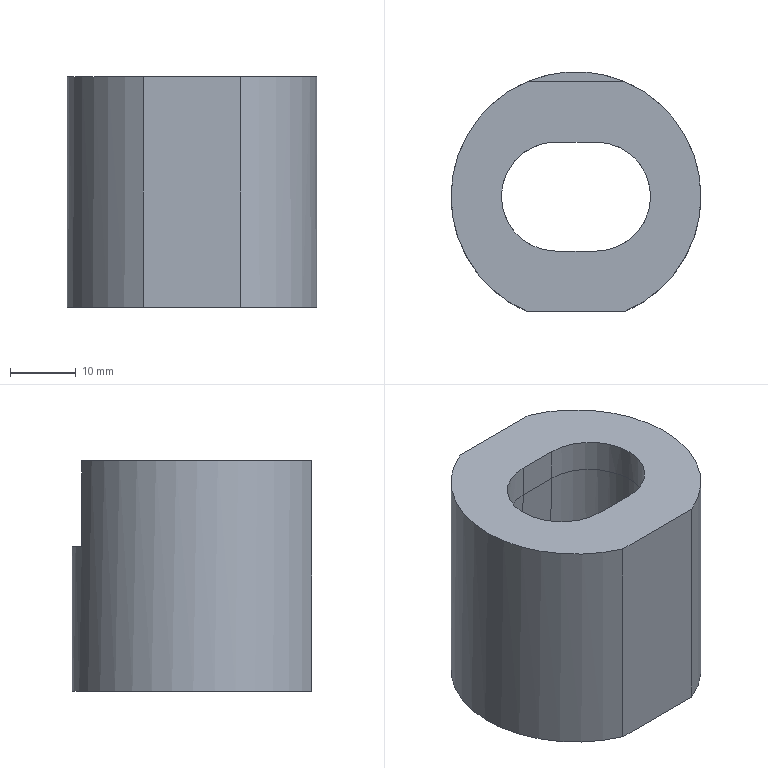Part | STEP file | 1_id4566_x_t | 1 solid | 14 faces | box 38 x 36.5 x 35 mm | volume 27105 mm3 | plane 9 | spline 4 | cylinder 1 | commonest cylinder face diameters 38 x1
STEP:
#1=CARTESIAN_POINT('',(3195.601,138.,-35.));
#2=VERTEX_POINT('',#1);
#3=CARTESIAN_POINT('',(3210.399,138.,-35.));
#4=VERTEX_POINT('',#3);
#5=CARTESIAN_POINT('',(3203.,138.,-35.));
#6=DIRECTION('',(1.,0.,0.));
#7=VECTOR('',#6,1.);
#8=LINE('',#5,#7);
#9=EDGE_CURVE('',#2,#4,#8,.T.);
#10=ORIENTED_EDGE('',*,*,#9,.F.);
#11=CARTESIAN_POINT('',(3203.,155.5,-35.));
#12=DIRECTION('',(0.,0.,1.));
#13=DIRECTION('',(-1.,0.,0.));
#14=AXIS2_PLACEMENT_3D('',#11,#12,#13);
#15=CIRCLE('',#14,19.);
#16=EDGE_CURVE('',#4,#2,#15,.T.);
#17=ORIENTED_EDGE('',*,*,#16,.F.);
#18=EDGE_LOOP('',(#10,#17));
#19=FACE_BOUND('',#18,.T.);
#20=CARTESIAN_POINT('',(3199.935,146.43,-35.));
#21=VERTEX_POINT('',#20);
#22=CARTESIAN_POINT('',(3199.935,164.571,-35.));
#23=VERTEX_POINT('',#22);
#24=CARTESIAN_POINT('',(3199.935,146.43,-35.));
#25=CARTESIAN_POINT('',(3197.549,146.43,-35.));
#26=CARTESIAN_POINT('',(3195.2,147.406,-35.));
#27=CARTESIAN_POINT('',(3191.84,150.768,-35.));
#28=CARTESIAN_POINT('',(3190.867,153.119,-35.));
#29=CARTESIAN_POINT('',(3190.862,157.866,-35.));
#30=CARTESIAN_POINT('',(3191.822,160.211,-35.));
#31=CARTESIAN_POINT('',(3195.207,163.604,-35.));
#32=CARTESIAN_POINT('',(3197.534,164.57,-35.));
#33=CARTESIAN_POINT('',(3199.935,164.571,-35.));
#34=CARTESIAN_POINT('',(3199.935,164.571,-35.));
#35=CARTESIAN_POINT('',(3199.935,164.571,-35.));
#36=B_SPLINE_CURVE_WITH_KNOTS('',3,(#24,#25,#26,#27,#28,#29,#30,#31,#32,#33,#34,#35),.UNSPECIFIED.,.F.,.F.,(4,2,2,2,2,4),(0.,0.25,0.5,0.75,1.,1.),.UNSPECIFIED.);
#37=EDGE_CURVE('',#21,#23,#36,.T.);
#38=ORIENTED_EDGE('',*,*,#37,.F.);
#39=CARTESIAN_POINT('',(3206.065,146.43,-35.));
#40=VERTEX_POINT('',#39);
#41=CARTESIAN_POINT('',(3203.,146.43,-35.));
#42=DIRECTION('',(-1.,0.,0.));
#43=VECTOR('',#42,1.);
#44=LINE('',#41,#43);
#45=EDGE_CURVE('',#40,#21,#44,.T.);
#46=ORIENTED_EDGE('',*,*,#45,.F.);
#47=CARTESIAN_POINT('',(3206.065,164.571,-35.));
#48=VERTEX_POINT('',#47);
#49=CARTESIAN_POINT('',(3206.065,164.571,-35.));
#50=CARTESIAN_POINT('',(3208.452,164.57,-35.));
#51=CARTESIAN_POINT('',(3210.8,163.594,-35.));
#52=CARTESIAN_POINT('',(3214.16,160.233,-35.));
#53=CARTESIAN_POINT('',(3215.134,157.881,-35.));
#54=CARTESIAN_POINT('',(3215.138,153.135,-35.));
#55=CARTESIAN_POINT('',(3214.178,150.789,-35.));
#56=CARTESIAN_POINT('',(3210.793,147.396,-35.));
#57=CARTESIAN_POINT('',(3208.466,146.43,-35.));
#58=CARTESIAN_POINT('',(3206.065,146.43,-35.));
#59=CARTESIAN_POINT('',(3206.065,146.43,-35.));
#60=CARTESIAN_POINT('',(3206.065,146.43,-35.));
#61=B_SPLINE_CURVE_WITH_KNOTS('',3,(#49,#50,#51,#52,#53,#54,#55,#56,#57,#58,#59,#60),.UNSPECIFIED.,.F.,.F.,(4,2,2,2,2,4),(0.,0.25,0.5,0.75,1.,1.),.UNSPECIFIED.);
#62=EDGE_CURVE('',#48,#40,#61,.T.);
#63=ORIENTED_EDGE('',*,*,#62,.F.);
#64=CARTESIAN_POINT('',(3203.,164.571,-35.));
#65=DIRECTION('',(1.,0.,0.));
#66=VECTOR('',#65,1.);
#67=LINE('',#64,#66);
#68=EDGE_CURVE('',#23,#48,#67,.T.);
#69=ORIENTED_EDGE('',*,*,#68,.F.);
#70=EDGE_LOOP('',(#38,#46,#63,#69));
#71=FACE_BOUND('',#70,.T.);
#72=CARTESIAN_POINT('',(3203.,161.75,-35.));
#73=DIRECTION('',(0.,0.,-1.));
#74=DIRECTION('',(0.,1.,0.));
#75=AXIS2_PLACEMENT_3D('',#72,#73,#74);
#76=PLANE('',#75);
#77=ADVANCED_FACE('',(#19,#71),#76,.T.);
#78=CARTESIAN_POINT('',(3195.601,173.,0.00001607));
#79=VERTEX_POINT('',#78);
#80=CARTESIAN_POINT('',(3210.399,173.,0.00001607));
#81=VERTEX_POINT('',#80);
#82=CARTESIAN_POINT('',(3550.42,173.,0.00001607));
#83=DIRECTION('',(1.,0.,0.));
#84=VECTOR('',#83,1.);
#85=LINE('',#82,#84);
#86=EDGE_CURVE('',#79,#81,#85,.T.);
#87=ORIENTED_EDGE('',*,*,#86,.F.);
#88=CARTESIAN_POINT('',(3195.601,138.,0.00001607));
#89=VERTEX_POINT('',#88);
#90=CARTESIAN_POINT('',(3203.,155.5,0.00001607));
#91=DIRECTION('',(0.,0.,1.));
#92=DIRECTION('',(1.,0.,0.));
#93=AXIS2_PLACEMENT_3D('',#90,#91,#92);
#94=CIRCLE('',#93,19.);
#95=EDGE_CURVE('',#79,#89,#94,.T.);
#96=ORIENTED_EDGE('',*,*,#95,.T.);
#97=CARTESIAN_POINT('',(3210.399,138.,0.00001607));
#98=VERTEX_POINT('',#97);
#99=CARTESIAN_POINT('',(3203.,138.,0.00001607));
#100=DIRECTION('',(-1.,0.,0.));
#101=VECTOR('',#100,1.);
#102=LINE('',#99,#101);
#103=EDGE_CURVE('',#98,#89,#102,.T.);
#104=ORIENTED_EDGE('',*,*,#103,.F.);
#105=CARTESIAN_POINT('',(3203.,155.5,0.00001607));
#106=DIRECTION('',(0.,0.,1.));
#107=DIRECTION('',(1.,0.,0.));
#108=AXIS2_PLACEMENT_3D('',#105,#106,#107);
#109=CIRCLE('',#108,19.);
#110=EDGE_CURVE('',#98,#81,#109,.T.);
#111=ORIENTED_EDGE('',*,*,#110,.T.);
#112=EDGE_LOOP('',(#87,#96,#104,#111));
#113=FACE_BOUND('',#112,.T.);
#114=CARTESIAN_POINT('',(3206.065,163.785,0.00001607));
#115=VERTEX_POINT('',#114);
#116=CARTESIAN_POINT('',(3206.065,147.215,0.00001607));
#117=VERTEX_POINT('',#116);
#118=CARTESIAN_POINT('',(3206.065,163.785,0.00001609));
#119=CARTESIAN_POINT('',(3206.589,163.785,0.00001609));
#120=CARTESIAN_POINT('',(3207.146,163.729,0.00001608));
#121=CARTESIAN_POINT('',(3208.207,163.514,0.00001607));
#122=CARTESIAN_POINT('',(3208.728,163.355,0.00001607));
#123=CARTESIAN_POINT('',(3210.231,162.733,0.00001606));
#124=CARTESIAN_POINT('',(3211.155,162.127,0.00001605));
#125=CARTESIAN_POINT('',(3213.46,159.822,0.00001604));
#126=CARTESIAN_POINT('',(3214.35,157.673,0.00001603));
#127=CARTESIAN_POINT('',(3214.35,153.328,0.00001603));
#128=CARTESIAN_POINT('',(3213.46,151.178,0.00001604));
#129=CARTESIAN_POINT('',(3210.387,148.105,0.00001606));
#130=CARTESIAN_POINT('',(3208.228,147.215,0.00001607));
#131=CARTESIAN_POINT('',(3206.065,147.215,0.00001609));
#132=B_SPLINE_CURVE_WITH_KNOTS('',3,(#118,#119,#120,#121,#122,#123,#124,#125,#126,#127,#128,#129,#130,#131),.UNSPECIFIED.,.F.,.F.,(4,2,2,2,2,2,4),(0.,0.0625,0.125,0.25,0.5,0.75,1.),.UNSPECIFIED.);
#133=EDGE_CURVE('',#115,#117,#132,.T.);
#134=ORIENTED_EDGE('',*,*,#133,.T.);
#135=CARTESIAN_POINT('',(3199.935,147.215,0.00001607));
#136=VERTEX_POINT('',#135);
#137=CARTESIAN_POINT('',(3203.,147.215,0.00001607));
#138=DIRECTION('',(-1.,0.,0.));
#139=VECTOR('',#138,1.);
#140=LINE('',#137,#139);
#141=EDGE_CURVE('',#117,#136,#140,.T.);
#142=ORIENTED_EDGE('',*,*,#141,.T.);
#143=CARTESIAN_POINT('',(3199.935,163.785,0.00001607));
#144=VERTEX_POINT('',#143);
#145=CARTESIAN_POINT('',(3199.935,147.215,0.00001607));
#146=CARTESIAN_POINT('',(3197.746,147.215,0.00001607));
#147=CARTESIAN_POINT('',(3195.599,148.119,0.00001607));
#148=CARTESIAN_POINT('',(3192.551,151.168,0.00001607));
#149=CARTESIAN_POINT('',(3191.652,153.333,0.00001607));
#150=CARTESIAN_POINT('',(3191.648,157.654,0.00001607));
#151=CARTESIAN_POINT('',(3192.53,159.809,0.00001607));
#152=CARTESIAN_POINT('',(3195.615,162.9,0.00001607));
#153=CARTESIAN_POINT('',(3197.747,163.785,0.00001607));
#154=CARTESIAN_POINT('',(3199.935,163.785,0.00001607));
#155=B_SPLINE_CURVE_WITH_KNOTS('',3,(#145,#146,#147,#148,#149,#150,#151,#152,#153,#154),.UNSPECIFIED.,.F.,.F.,(4,2,2,2,4),(0.,0.25,0.5,0.75,1.),.UNSPECIFIED.);
#156=EDGE_CURVE('',#136,#144,#155,.T.);
#157=ORIENTED_EDGE('',*,*,#156,.T.);
#158=CARTESIAN_POINT('',(3203.,163.785,0.00001607));
#159=DIRECTION('',(1.,0.,0.));
#160=VECTOR('',#159,1.);
#161=LINE('',#158,#160);
#162=EDGE_CURVE('',#144,#115,#161,.T.);
#163=ORIENTED_EDGE('',*,*,#162,.T.);
#164=EDGE_LOOP('',(#134,#142,#157,#163));
#165=FACE_BOUND('',#164,.T.);
#166=CARTESIAN_POINT('',(3203.,161.75,0.00001607));
#167=DIRECTION('',(0.,0.,1.));
#168=DIRECTION('',(0.,-1.,0.));
#169=AXIS2_PLACEMENT_3D('',#166,#167,#168);
#170=PLANE('',#169);
#171=ADVANCED_FACE('',(#113,#165),#170,.T.);
#172=ORIENTED_EDGE('',*,*,#95,.F.);
#173=CARTESIAN_POINT('',(3195.601,173.,-13.));
#174=VERTEX_POINT('',#173);
#175=CARTESIAN_POINT('',(3195.601,173.,-17.5));
#176=DIRECTION('',(0.,0.,-1.));
#177=VECTOR('',#176,1.);
#178=LINE('',#175,#177);
#179=EDGE_CURVE('',#79,#174,#178,.T.);
#180=ORIENTED_EDGE('',*,*,#179,.T.);
#181=CARTESIAN_POINT('',(3210.399,173.,-13.));
#182=VERTEX_POINT('',#181);
#183=CARTESIAN_POINT('',(3203.,155.5,-13.));
#184=DIRECTION('',(0.,0.,-1.));
#185=DIRECTION('',(1.,0.,0.));
#186=AXIS2_PLACEMENT_3D('',#183,#184,#185);
#187=CIRCLE('',#186,19.);
#188=EDGE_CURVE('',#174,#182,#187,.T.);
#189=ORIENTED_EDGE('',*,*,#188,.T.);
#190=CARTESIAN_POINT('',(3210.399,173.,-17.5));
#191=DIRECTION('',(0.,0.,1.));
#192=VECTOR('',#191,1.);
#193=LINE('',#190,#192);
#194=EDGE_CURVE('',#182,#81,#193,.T.);
#195=ORIENTED_EDGE('',*,*,#194,.T.);
#196=ORIENTED_EDGE('',*,*,#110,.F.);
#197=CARTESIAN_POINT('',(3210.399,138.,-17.5));
#198=DIRECTION('',(0.,0.,1.));
#199=VECTOR('',#198,1.);
#200=LINE('',#197,#199);
#201=EDGE_CURVE('',#4,#98,#200,.T.);
#202=ORIENTED_EDGE('',*,*,#201,.F.);
#203=ORIENTED_EDGE('',*,*,#16,.T.);
#204=CARTESIAN_POINT('',(3195.601,138.,-17.5));
#205=DIRECTION('',(0.,0.,-1.));
#206=VECTOR('',#205,1.);
#207=LINE('',#204,#206);
#208=EDGE_CURVE('',#89,#2,#207,.T.);
#209=ORIENTED_EDGE('',*,*,#208,.F.);
#210=EDGE_LOOP('',(#172,#180,#189,#195,#196,#202,#203,#209));
#211=FACE_OUTER_BOUND('',#210,.T.);
#212=CARTESIAN_POINT('',(3203.,155.5,-17.5));
#213=DIRECTION('',(0.,0.,1.));
#214=DIRECTION('',(0.,-1.,0.));
#215=AXIS2_PLACEMENT_3D('',#212,#213,#214);
#216=CYLINDRICAL_SURFACE('',#215,19.);
#217=ADVANCED_FACE('',(#211),#216,.T.);
#218=CARTESIAN_POINT('',(3199.935,163.785,-5.));
#219=VERTEX_POINT('',#218);
#220=CARTESIAN_POINT('',(3206.065,163.785,-5.));
#221=VERTEX_POINT('',#220);
#222=CARTESIAN_POINT('',(3199.935,163.785,-5.));
#223=DIRECTION('',(1.,0.,0.));
#224=VECTOR('',#223,1.);
#225=LINE('',#222,#224);
#226=EDGE_CURVE('',#219,#221,#225,.T.);
#227=ORIENTED_EDGE('',*,*,#226,.T.);
#228=CARTESIAN_POINT('',(3206.065,163.785,0.00001605));
#229=DIRECTION('',(0.000000008,0.,1.));
#230=VECTOR('',#229,1.);
#231=LINE('',#228,#230);
#232=EDGE_CURVE('',#221,#115,#231,.T.);
#233=ORIENTED_EDGE('',*,*,#232,.T.);
#234=ORIENTED_EDGE('',*,*,#162,.F.);
#235=CARTESIAN_POINT('',(3199.935,163.785,0.0000161));
#236=DIRECTION('',(0.000000008,0.,1.));
#237=VECTOR('',#236,1.);
#238=LINE('',#235,#237);
#239=EDGE_CURVE('',#219,#144,#238,.T.);
#240=ORIENTED_EDGE('',*,*,#239,.F.);
#241=EDGE_LOOP('',(#227,#233,#234,#240));
#242=FACE_OUTER_BOUND('',#241,.T.);
#243=CARTESIAN_POINT('',(3192.,163.785,0.00001616));
#244=DIRECTION('',(0.,-1.,0.));
#245=DIRECTION('',(1.,0.,-0.000000008));
#246=AXIS2_PLACEMENT_3D('',#243,#244,#245);
#247=PLANE('',#246);
#248=ADVANCED_FACE('',(#242),#247,.T.);
#249=CARTESIAN_POINT('',(3199.935,147.215,-5.));
#250=VERTEX_POINT('',#249);
#251=CARTESIAN_POINT('',(3199.926,147.215,-5.));
#252=VERTEX_POINT('',#251);
#253=CARTESIAN_POINT('',(3199.935,147.215,-5.));
#254=CARTESIAN_POINT('',(3199.932,147.215,-5.));
#255=CARTESIAN_POINT('',(3199.929,147.215,-5.));
#256=CARTESIAN_POINT('',(3199.926,147.215,-5.));
#257=B_SPLINE_CURVE_WITH_KNOTS('',3,(#253,#254,#255,#256),.UNSPECIFIED.,.F.,.F.,(4,4),(0.,1.),.UNSPECIFIED.);
#258=EDGE_CURVE('',#250,#252,#257,.T.);
#259=ORIENTED_EDGE('',*,*,#258,.T.);
#260=CARTESIAN_POINT('',(3191.65,155.494,-5.));
#261=VERTEX_POINT('',#260);
#262=CARTESIAN_POINT('',(3199.926,147.215,-5.));
#263=CARTESIAN_POINT('',(3199.334,147.216,-5.));
#264=CARTESIAN_POINT('',(3198.392,147.278,-5.));
#265=CARTESIAN_POINT('',(3196.68,147.868,-5.));
#266=CARTESIAN_POINT('',(3196.057,148.15,-5.));
#267=CARTESIAN_POINT('',(3195.108,148.761,-4.999));
#268=CARTESIAN_POINT('',(3194.76,149.023,-4.999));
#269=CARTESIAN_POINT('',(3194.234,149.478,-5.001));
#270=CARTESIAN_POINT('',(3194.035,149.68,-5.002));
#271=CARTESIAN_POINT('',(3193.741,149.995,-5.007));
#272=CARTESIAN_POINT('',(3193.686,150.057,-5.008));
#273=CARTESIAN_POINT('',(3193.424,150.375,-5.023));
#274=CARTESIAN_POINT('',(3193.266,150.573,-5.034));
#275=CARTESIAN_POINT('',(3192.828,151.234,-5.073));
#276=CARTESIAN_POINT('',(3192.686,151.495,-5.087));
#277=CARTESIAN_POINT('',(3192.505,151.844,-5.101));
#278=CARTESIAN_POINT('',(3192.403,152.055,-5.105));
#279=CARTESIAN_POINT('',(3192.206,152.525,-5.104));
#280=CARTESIAN_POINT('',(3192.111,152.779,-5.099));
#281=CARTESIAN_POINT('',(3191.983,153.192,-5.086));
#282=CARTESIAN_POINT('',(3191.942,153.335,-5.08));
#283=CARTESIAN_POINT('',(3191.867,153.63,-5.067));
#284=CARTESIAN_POINT('',(3191.818,153.85,-5.056));
#285=CARTESIAN_POINT('',(3191.652,154.752,-5.016));
#286=CARTESIAN_POINT('',(3191.65,155.247,-5.));
#287=CARTESIAN_POINT('',(3191.65,155.494,-5.));
#288=B_SPLINE_CURVE_WITH_KNOTS('',3,(#262,#263,#264,#265,#266,#267,#268,#269,#270,#271,#272,#273,#274,#275,#276,#277,#278,#279,#280,#281,#282,#283,#284,#285,#286,#287),.UNSPECIFIED.,.F.,.F.,(4,2,2,2,2,2,2,2,2,2,2,2,4),(0.,0.25,0.375,0.4375,0.5,0.5625,0.625,0.6875,0.75,0.8125,0.8437,0.875,1.),.UNSPECIFIED.);
#289=EDGE_CURVE('',#252,#261,#288,.T.);
#290=ORIENTED_EDGE('',*,*,#289,.T.);
#291=CARTESIAN_POINT('',(3191.991,157.831,-5.));
#292=VERTEX_POINT('',#291);
#293=CARTESIAN_POINT('',(3191.65,155.494,-5.));
#294=CARTESIAN_POINT('',(3191.65,155.496,-5.));
#295=CARTESIAN_POINT('',(3191.65,155.498,-5.));
#296=CARTESIAN_POINT('',(3191.65,156.289,-5.));
#297=CARTESIAN_POINT('',(3191.767,157.076,-5.));
#298=CARTESIAN_POINT('',(3191.991,157.831,-5.));
#299=B_SPLINE_CURVE_WITH_KNOTS('',3,(#293,#294,#295,#296,#297,#298),.UNSPECIFIED.,.F.,.F.,(4,2,4),(0.,0.002603,1.),.UNSPECIFIED.);
#300=EDGE_CURVE('',#261,#292,#299,.T.);
#301=ORIENTED_EDGE('',*,*,#300,.T.);
#302=CARTESIAN_POINT('',(3194.07,161.352,-5.));
#303=VERTEX_POINT('',#302);
#304=CARTESIAN_POINT('',(3191.991,157.831,-5.));
#305=CARTESIAN_POINT('',(3192.381,159.151,-5.));
#306=CARTESIAN_POINT('',(3193.095,160.375,-5.));
#307=CARTESIAN_POINT('',(3194.07,161.352,-5.));
#308=B_SPLINE_CURVE_WITH_KNOTS('',3,(#304,#305,#306,#307),.UNSPECIFIED.,.F.,.F.,(4,4),(0.,1.),.UNSPECIFIED.);
#309=EDGE_CURVE('',#292,#303,#308,.T.);
#310=ORIENTED_EDGE('',*,*,#309,.T.);
#311=CARTESIAN_POINT('',(3199.926,163.785,-5.));
#312=VERTEX_POINT('',#311);
#313=CARTESIAN_POINT('',(3194.07,161.352,-5.));
#314=CARTESIAN_POINT('',(3194.072,161.354,-5.));
#315=CARTESIAN_POINT('',(3194.074,161.356,-5.));
#316=CARTESIAN_POINT('',(3194.845,162.127,-5.));
#317=CARTESIAN_POINT('',(3195.769,162.733,-5.));
#318=CARTESIAN_POINT('',(3197.272,163.355,-5.));
#319=CARTESIAN_POINT('',(3197.793,163.514,-5.));
#320=CARTESIAN_POINT('',(3198.851,163.729,-5.));
#321=CARTESIAN_POINT('',(3199.405,163.784,-5.));
#322=CARTESIAN_POINT('',(3199.926,163.785,-5.));
#323=B_SPLINE_CURVE_WITH_KNOTS('',3,(#313,#314,#315,#316,#317,#318,#319,#320,#321,#322),.UNSPECIFIED.,.F.,.F.,(4,2,2,2,4),(0.,0.001413,0.5014,0.7514,1.),.UNSPECIFIED.);
#324=EDGE_CURVE('',#303,#312,#323,.T.);
#325=ORIENTED_EDGE('',*,*,#324,.T.);
#326=CARTESIAN_POINT('',(3199.926,163.785,-5.));
#327=CARTESIAN_POINT('',(3199.929,163.785,-5.));
#328=CARTESIAN_POINT('',(3199.932,163.785,-5.));
#329=CARTESIAN_POINT('',(3199.935,163.785,-5.));
#330=B_SPLINE_CURVE_WITH_KNOTS('',3,(#326,#327,#328,#329),.UNSPECIFIED.,.F.,.F.,(4,4),(0.,1.),.UNSPECIFIED.);
#331=EDGE_CURVE('',#312,#219,#330,.T.);
#332=ORIENTED_EDGE('',*,*,#331,.T.);
#333=ORIENTED_EDGE('',*,*,#239,.T.);
#334=ORIENTED_EDGE('',*,*,#156,.F.);
#335=CARTESIAN_POINT('',(3199.935,147.215,0.00001609));
#336=DIRECTION('',(0.000000008,0.,1.));
#337=VECTOR('',#336,1.);
#338=LINE('',#335,#337);
#339=EDGE_CURVE('',#250,#136,#338,.T.);
#340=ORIENTED_EDGE('',*,*,#339,.F.);
#341=EDGE_LOOP('',(#259,#290,#301,#310,#325,#332,#333,#334,#340));
#342=FACE_OUTER_BOUND('',#341,.T.);
#343=CARTESIAN_POINT('',(3199.935,147.215,-5.146));
#344=CARTESIAN_POINT('',(3199.935,147.215,0.00001607));
#345=CARTESIAN_POINT('',(3199.411,147.215,-5.146));
#346=CARTESIAN_POINT('',(3199.411,147.215,0.00001608));
#347=CARTESIAN_POINT('',(3198.854,147.271,-5.146));
#348=CARTESIAN_POINT('',(3198.854,147.271,0.00001608));
#349=CARTESIAN_POINT('',(3197.793,147.486,-5.146));
#350=CARTESIAN_POINT('',(3197.793,147.486,0.00001609));
#351=CARTESIAN_POINT('',(3197.272,147.646,-5.146));
#352=CARTESIAN_POINT('',(3197.272,147.646,0.00001609));
#353=CARTESIAN_POINT('',(3195.769,148.267,-5.146));
#354=CARTESIAN_POINT('',(3195.769,148.267,0.0000161));
#355=CARTESIAN_POINT('',(3194.845,148.873,-5.146));
#356=CARTESIAN_POINT('',(3194.845,148.873,0.00001611));
#357=CARTESIAN_POINT('',(3192.54,151.178,-5.146));
#358=CARTESIAN_POINT('',(3192.54,151.178,0.00001613));
#359=CARTESIAN_POINT('',(3191.65,153.327,-5.146));
#360=CARTESIAN_POINT('',(3191.65,153.327,0.00001614));
#361=CARTESIAN_POINT('',(3191.65,157.673,-5.146));
#362=CARTESIAN_POINT('',(3191.65,157.673,0.00001614));
#363=CARTESIAN_POINT('',(3192.54,159.822,-5.146));
#364=CARTESIAN_POINT('',(3192.54,159.822,0.00001613));
#365=CARTESIAN_POINT('',(3194.845,162.127,-5.146));
#366=CARTESIAN_POINT('',(3194.845,162.127,0.00001611));
#367=CARTESIAN_POINT('',(3195.769,162.733,-5.146));
#368=CARTESIAN_POINT('',(3195.769,162.733,0.0000161));
#369=CARTESIAN_POINT('',(3197.272,163.355,-5.146));
#370=CARTESIAN_POINT('',(3197.272,163.355,0.00001609));
#371=CARTESIAN_POINT('',(3197.793,163.514,-5.146));
#372=CARTESIAN_POINT('',(3197.793,163.514,0.00001609));
#373=CARTESIAN_POINT('',(3198.854,163.729,-5.146));
#374=CARTESIAN_POINT('',(3198.854,163.729,0.00001608));
#375=CARTESIAN_POINT('',(3199.411,163.785,-5.146));
#376=CARTESIAN_POINT('',(3199.411,163.785,0.00001608));
#377=CARTESIAN_POINT('',(3199.935,163.785,-5.146));
#378=CARTESIAN_POINT('',(3199.935,163.785,0.00001607));
#379=B_SPLINE_SURFACE_WITH_KNOTS('',3,1,((#343,#344),(#345,#346),(#347,#348),(#349,#350),(#351,#352),(#353,#354),(#355,#356),(#357,#358),(#359,#360),(#361,#362),(#363,#364),(#365,#366),(#367,#368),(#369,#370),(#371,#372),(#373,#374),(#375,#376),(#377,#378)),.UNSPECIFIED.,.F.,.F.,.F.,(4,2,2,2,2,2,2,2,4),(2,2),(0.,0.0625,0.125,0.25,0.5,0.75,0.875,0.9375,1.),(0.,1.),.UNSPECIFIED.);
#380=ADVANCED_FACE('',(#342),#379,.T.);
#381=CARTESIAN_POINT('',(3206.075,163.785,-5.));
#382=VERTEX_POINT('',#381);
#383=CARTESIAN_POINT('',(3206.07,163.785,-5.));
#384=DIRECTION('',(1.,-0.0001546,0.));
#385=VECTOR('',#384,1.);
#386=LINE('',#383,#385);
#387=EDGE_CURVE('',#221,#382,#386,.T.);
#388=ORIENTED_EDGE('',*,*,#387,.T.);
#389=CARTESIAN_POINT('',(3214.35,155.507,-5.));
#390=VERTEX_POINT('',#389);
#391=CARTESIAN_POINT('',(3206.075,163.785,-5.));
#392=CARTESIAN_POINT('',(3208.263,163.782,-5.));
#393=CARTESIAN_POINT('',(3210.406,162.88,-4.999));
#394=CARTESIAN_POINT('',(3212.692,160.588,-5.001));
#395=CARTESIAN_POINT('',(3213.3,159.663,-5.107));
#396=CARTESIAN_POINT('',(3214.125,157.671,-5.107));
#397=CARTESIAN_POINT('',(3214.349,156.587,-5.));
#398=CARTESIAN_POINT('',(3214.35,155.507,-5.));
#399=B_SPLINE_CURVE_WITH_KNOTS('',3,(#391,#392,#393,#394,#395,#396,#397,#398),.UNSPECIFIED.,.F.,.F.,(4,2,2,4),(0.,0.5,0.75,1.),.UNSPECIFIED.);
#400=EDGE_CURVE('',#382,#390,#399,.T.);
#401=ORIENTED_EDGE('',*,*,#400,.T.);
#402=CARTESIAN_POINT('',(3214.35,155.506,-5.));
#403=VERTEX_POINT('',#402);
#404=CARTESIAN_POINT('',(3214.35,155.507,-5.));
#405=CARTESIAN_POINT('',(3214.35,155.507,-5.));
#406=CARTESIAN_POINT('',(3214.35,155.507,-5.));
#407=CARTESIAN_POINT('',(3214.35,155.506,-5.));
#408=B_SPLINE_CURVE_WITH_KNOTS('',3,(#404,#405,#406,#407),.UNSPECIFIED.,.F.,.F.,(4,4),(0.,1.),.UNSPECIFIED.);
#409=EDGE_CURVE('',#390,#403,#408,.T.);
#410=ORIENTED_EDGE('',*,*,#409,.T.);
#411=CARTESIAN_POINT('',(3214.009,153.171,-5.));
#412=VERTEX_POINT('',#411);
#413=CARTESIAN_POINT('',(3214.35,155.506,-5.));
#414=CARTESIAN_POINT('',(3214.351,154.715,-5.));
#415=CARTESIAN_POINT('',(3214.233,153.926,-5.002));
#416=CARTESIAN_POINT('',(3214.01,153.17,-5.));
#417=B_SPLINE_CURVE_WITH_KNOTS('',3,(#413,#414,#415,#416),.UNSPECIFIED.,.F.,.F.,(4,4),(0.,1.),.UNSPECIFIED.);
#418=EDGE_CURVE('',#403,#412,#417,.T.);
#419=ORIENTED_EDGE('',*,*,#418,.T.);
#420=CARTESIAN_POINT('',(3211.93,149.648,-5.));
#421=VERTEX_POINT('',#420);
#422=CARTESIAN_POINT('',(3214.01,153.17,-5.));
#423=CARTESIAN_POINT('',(3213.619,151.85,-5.));
#424=CARTESIAN_POINT('',(3212.905,150.626,-5.));
#425=CARTESIAN_POINT('',(3211.93,149.648,-5.));
#426=B_SPLINE_CURVE_WITH_KNOTS('',3,(#422,#423,#424,#425),.UNSPECIFIED.,.F.,.F.,(4,4),(0.,1.),.UNSPECIFIED.);
#427=EDGE_CURVE('',#412,#421,#426,.T.);
#428=ORIENTED_EDGE('',*,*,#427,.T.);
#429=CARTESIAN_POINT('',(3206.074,147.215,-5.));
#430=VERTEX_POINT('',#429);
#431=CARTESIAN_POINT('',(3211.93,149.648,-5.));
#432=CARTESIAN_POINT('',(3211.928,149.646,-5.));
#433=CARTESIAN_POINT('',(3211.926,149.644,-5.));
#434=CARTESIAN_POINT('',(3210.389,148.108,-5.));
#435=CARTESIAN_POINT('',(3208.234,147.218,-5.));
#436=CARTESIAN_POINT('',(3206.074,147.215,-5.));
#437=B_SPLINE_CURVE_WITH_KNOTS('',3,(#431,#432,#433,#434,#435,#436),.UNSPECIFIED.,.F.,.F.,(4,2,4),(0.,0.00141,1.),.UNSPECIFIED.);
#438=EDGE_CURVE('',#421,#430,#437,.T.);
#439=ORIENTED_EDGE('',*,*,#438,.T.);
#440=CARTESIAN_POINT('',(3206.065,147.215,-5.));
#441=VERTEX_POINT('',#440);
#442=CARTESIAN_POINT('',(3206.074,147.215,-5.));
#443=CARTESIAN_POINT('',(3206.071,147.215,-5.));
#444=CARTESIAN_POINT('',(3206.068,147.215,-5.));
#445=CARTESIAN_POINT('',(3206.065,147.215,-5.));
#446=B_SPLINE_CURVE_WITH_KNOTS('',3,(#442,#443,#444,#445),.UNSPECIFIED.,.F.,.F.,(4,4),(0.,1.),.UNSPECIFIED.);
#447=EDGE_CURVE('',#430,#441,#446,.T.);
#448=ORIENTED_EDGE('',*,*,#447,.T.);
#449=CARTESIAN_POINT('',(3206.065,147.215,0.00001605));
#450=DIRECTION('',(0.000000008,0.,1.));
#451=VECTOR('',#450,1.);
#452=LINE('',#449,#451);
#453=EDGE_CURVE('',#441,#117,#452,.T.);
#454=ORIENTED_EDGE('',*,*,#453,.T.);
#455=ORIENTED_EDGE('',*,*,#133,.F.);
#456=ORIENTED_EDGE('',*,*,#232,.F.);
#457=EDGE_LOOP('',(#388,#401,#410,#419,#428,#439,#448,#454,#455,#456));
#458=FACE_OUTER_BOUND('',#457,.T.);
#459=CARTESIAN_POINT('',(3206.065,163.785,-5.146));
#460=CARTESIAN_POINT('',(3206.065,163.785,0.0000161));
#461=CARTESIAN_POINT('',(3206.589,163.785,-5.146));
#462=CARTESIAN_POINT('',(3206.589,163.785,0.0000161));
#463=CARTESIAN_POINT('',(3207.146,163.729,-5.146));
#464=CARTESIAN_POINT('',(3207.146,163.729,0.0000161));
#465=CARTESIAN_POINT('',(3208.207,163.514,-5.146));
#466=CARTESIAN_POINT('',(3208.207,163.514,0.00001609));
#467=CARTESIAN_POINT('',(3208.728,163.355,-5.146));
#468=CARTESIAN_POINT('',(3208.728,163.355,0.00001608));
#469=CARTESIAN_POINT('',(3210.231,162.733,-5.146));
#470=CARTESIAN_POINT('',(3210.231,162.733,0.00001607));
#471=CARTESIAN_POINT('',(3211.155,162.127,-5.146));
#472=CARTESIAN_POINT('',(3211.155,162.127,0.00001607));
#473=CARTESIAN_POINT('',(3213.46,159.822,-5.146));
#474=CARTESIAN_POINT('',(3213.46,159.822,0.00001605));
#475=CARTESIAN_POINT('',(3214.35,157.673,-5.146));
#476=CARTESIAN_POINT('',(3214.35,157.673,0.00001604));
#477=CARTESIAN_POINT('',(3214.35,153.328,-5.146));
#478=CARTESIAN_POINT('',(3214.35,153.328,0.00001604));
#479=CARTESIAN_POINT('',(3213.46,151.178,-5.146));
#480=CARTESIAN_POINT('',(3213.46,151.178,0.00001605));
#481=CARTESIAN_POINT('',(3210.387,148.105,-5.146));
#482=CARTESIAN_POINT('',(3210.387,148.105,0.00001607));
#483=CARTESIAN_POINT('',(3208.228,147.215,-5.146));
#484=CARTESIAN_POINT('',(3208.228,147.215,0.00001609));
#485=CARTESIAN_POINT('',(3206.065,147.215,-5.146));
#486=CARTESIAN_POINT('',(3206.065,147.215,0.0000161));
#487=B_SPLINE_SURFACE_WITH_KNOTS('',3,1,((#459,#460),(#461,#462),(#463,#464),(#465,#466),(#467,#468),(#469,#470),(#471,#472),(#473,#474),(#475,#476),(#477,#478),(#479,#480),(#481,#482),(#483,#484),(#485,#486)),.UNSPECIFIED.,.F.,.F.,.F.,(4,2,2,2,2,2,4),(2,2),(0.,0.0625,0.125,0.25,0.5,0.75,1.),(0.,1.),.UNSPECIFIED.);
#488=ADVANCED_FACE('',(#458),#487,.T.);
#489=CARTESIAN_POINT('',(3206.065,147.215,-5.));
#490=DIRECTION('',(-1.,0.,0.));
#491=VECTOR('',#490,1.);
#492=LINE('',#489,#491);
#493=EDGE_CURVE('',#441,#250,#492,.T.);
#494=ORIENTED_EDGE('',*,*,#493,.T.);
#495=ORIENTED_EDGE('',*,*,#339,.T.);
#496=ORIENTED_EDGE('',*,*,#141,.F.);
#497=ORIENTED_EDGE('',*,*,#453,.F.);
#498=EDGE_LOOP('',(#494,#495,#496,#497));
#499=FACE_OUTER_BOUND('',#498,.T.);
#500=CARTESIAN_POINT('',(3192.,147.215,0.00001615));
#501=DIRECTION('',(0.,1.,0.));
#502=DIRECTION('',(-1.,0.,0.000000008));
#503=AXIS2_PLACEMENT_3D('',#500,#501,#502);
#504=PLANE('',#503);
#505=ADVANCED_FACE('',(#499),#504,.T.);
#506=ORIENTED_EDGE('',*,*,#208,.T.);
#507=ORIENTED_EDGE('',*,*,#9,.T.);
#508=ORIENTED_EDGE('',*,*,#201,.T.);
#509=ORIENTED_EDGE('',*,*,#103,.T.);
#510=EDGE_LOOP('',(#506,#507,#508,#509));
#511=FACE_OUTER_BOUND('',#510,.T.);
#512=CARTESIAN_POINT('',(3187.075,138.,-17.5));
#513=DIRECTION('',(0.,1.,0.));
#514=DIRECTION('',(-1.,0.,0.));
#515=AXIS2_PLACEMENT_3D('',#512,#513,#514);
#516=PLANE('',#515);
#517=ADVANCED_FACE('',(#511),#516,.F.);
#518=ORIENTED_EDGE('',*,*,#37,.T.);
#519=CARTESIAN_POINT('',(3199.935,163.785,-5.));
#520=DIRECTION('',(0.,0.02618,-0.9997));
#521=VECTOR('',#520,1.);
#522=LINE('',#519,#521);
#523=EDGE_CURVE('',#219,#23,#522,.T.);
#524=ORIENTED_EDGE('',*,*,#523,.F.);
#525=ORIENTED_EDGE('',*,*,#331,.F.);
#526=ORIENTED_EDGE('',*,*,#324,.F.);
#527=ORIENTED_EDGE('',*,*,#309,.F.);
#528=ORIENTED_EDGE('',*,*,#300,.F.);
#529=ORIENTED_EDGE('',*,*,#289,.F.);
#530=ORIENTED_EDGE('',*,*,#258,.F.);
#531=CARTESIAN_POINT('',(3199.935,147.215,-5.));
#532=DIRECTION('',(-0.000004048,-0.02618,-0.9997));
#533=VECTOR('',#532,1.);
#534=LINE('',#531,#533);
#535=EDGE_CURVE('',#250,#21,#534,.T.);
#536=ORIENTED_EDGE('',*,*,#535,.T.);
#537=EDGE_LOOP('',(#518,#524,#525,#526,#527,#528,#529,#530,#536));
#538=FACE_OUTER_BOUND('',#537,.T.);
#539=CARTESIAN_POINT('',(3199.935,147.226,-4.58));
#540=CARTESIAN_POINT('',(3197.768,147.226,-4.58));
#541=CARTESIAN_POINT('',(3195.608,148.125,-4.58));
#542=CARTESIAN_POINT('',(3192.559,151.175,-4.58));
#543=CARTESIAN_POINT('',(3191.663,153.339,-4.58));
#544=CARTESIAN_POINT('',(3191.659,157.647,-4.58));
#545=CARTESIAN_POINT('',(3192.538,159.801,-4.58));
#546=CARTESIAN_POINT('',(3195.619,162.889,-4.58));
#547=CARTESIAN_POINT('',(3197.749,163.774,-4.58));
#548=CARTESIAN_POINT('',(3200.022,163.774,-4.58));
#549=CARTESIAN_POINT('',(3200.11,163.774,-4.58));
#550=CARTESIAN_POINT('',(3200.197,163.774,-4.58));
#551=CARTESIAN_POINT('',(3199.935,147.215,-5.));
#552=CARTESIAN_POINT('',(3197.765,147.215,-5.));
#553=CARTESIAN_POINT('',(3195.602,148.115,-5.));
#554=CARTESIAN_POINT('',(3192.549,151.169,-5.));
#555=CARTESIAN_POINT('',(3191.652,153.336,-5.));
#556=CARTESIAN_POINT('',(3191.648,157.65,-5.));
#557=CARTESIAN_POINT('',(3192.528,159.807,-5.));
#558=CARTESIAN_POINT('',(3195.613,162.898,-5.));
#559=CARTESIAN_POINT('',(3197.746,163.785,-5.));
#560=CARTESIAN_POINT('',(3200.023,163.785,-5.));
#561=CARTESIAN_POINT('',(3200.11,163.785,-5.));
#562=CARTESIAN_POINT('',(3200.198,163.785,-5.));
#563=CARTESIAN_POINT('',(3199.935,146.115,-47.));
#564=CARTESIAN_POINT('',(3197.462,146.116,-47.));
#565=CARTESIAN_POINT('',(3195.04,147.123,-47.));
#566=CARTESIAN_POINT('',(3191.557,150.607,-47.));
#567=CARTESIAN_POINT('',(3190.552,153.032,-47.));
#568=CARTESIAN_POINT('',(3190.548,157.952,-47.));
#569=CARTESIAN_POINT('',(3191.539,160.373,-47.));
#570=CARTESIAN_POINT('',(3195.045,163.886,-47.));
#571=CARTESIAN_POINT('',(3197.45,164.885,-47.));
#572=CARTESIAN_POINT('',(3200.034,164.885,-47.));
#573=CARTESIAN_POINT('',(3200.134,164.885,-47.));
#574=CARTESIAN_POINT('',(3200.233,164.885,-47.));
#575=B_SPLINE_SURFACE_WITH_KNOTS('',1,3,((#539,#540,#541,#542,#543,#544,#545,#546,#547,#548,#549,#550),(#551,#552,#553,#554,#555,#556,#557,#558,#559,#560,#561,#562),(#563,#564,#565,#566,#567,#568,#569,#570,#571,#572,#573,#574)),.UNSPECIFIED.,.F.,.F.,.F.,(2,1,2),(4,2,2,2,2,4),(0.,0.009901,1.),(0.,0.2475,0.495,0.7426,0.9901,1.),.UNSPECIFIED.);
#576=ADVANCED_FACE('',(#538),#575,.T.);
#577=ORIENTED_EDGE('',*,*,#68,.T.);
#578=CARTESIAN_POINT('',(3206.065,163.785,-5.));
#579=DIRECTION('',(0.000004048,0.02618,-0.9997));
#580=VECTOR('',#579,1.);
#581=LINE('',#578,#580);
#582=EDGE_CURVE('',#221,#48,#581,.T.);
#583=ORIENTED_EDGE('',*,*,#582,.F.);
#584=ORIENTED_EDGE('',*,*,#226,.F.);
#585=ORIENTED_EDGE('',*,*,#523,.T.);
#586=EDGE_LOOP('',(#577,#583,#584,#585));
#587=FACE_OUTER_BOUND('',#586,.T.);
#588=CARTESIAN_POINT('',(3199.935,163.785,-5.));
#589=DIRECTION('',(0.,-0.9997,-0.02618));
#590=DIRECTION('',(0.,0.02618,-0.9997));
#591=AXIS2_PLACEMENT_3D('',#588,#589,#590);
#592=PLANE('',#591);
#593=ADVANCED_FACE('',(#587),#592,.T.);
#594=ORIENTED_EDGE('',*,*,#62,.T.);
#595=CARTESIAN_POINT('',(3206.065,147.215,-5.));
#596=DIRECTION('',(0.,-0.02618,-0.9997));
#597=VECTOR('',#596,1.);
#598=LINE('',#595,#597);
#599=EDGE_CURVE('',#441,#40,#598,.T.);
#600=ORIENTED_EDGE('',*,*,#599,.F.);
#601=ORIENTED_EDGE('',*,*,#447,.F.);
#602=ORIENTED_EDGE('',*,*,#438,.F.);
#603=ORIENTED_EDGE('',*,*,#427,.F.);
#604=ORIENTED_EDGE('',*,*,#418,.F.);
#605=ORIENTED_EDGE('',*,*,#409,.F.);
#606=ORIENTED_EDGE('',*,*,#400,.F.);
#607=ORIENTED_EDGE('',*,*,#387,.F.);
#608=ORIENTED_EDGE('',*,*,#582,.T.);
#609=EDGE_LOOP('',(#594,#600,#601,#602,#603,#604,#605,#606,#607,#608));
#610=FACE_OUTER_BOUND('',#609,.T.);
#611=CARTESIAN_POINT('',(3206.065,163.785,-5.));
#612=CARTESIAN_POINT('',(3208.236,163.785,-5.));
#613=CARTESIAN_POINT('',(3210.398,162.885,-5.));
#614=CARTESIAN_POINT('',(3213.451,159.831,-5.));
#615=CARTESIAN_POINT('',(3214.348,157.664,-5.));
#616=CARTESIAN_POINT('',(3214.352,153.351,-5.));
#617=CARTESIAN_POINT('',(3213.472,151.194,-5.));
#618=CARTESIAN_POINT('',(3210.387,148.102,-5.));
#619=CARTESIAN_POINT('',(3208.254,147.215,-5.));
#620=CARTESIAN_POINT('',(3205.978,147.215,-5.));
#621=CARTESIAN_POINT('',(3205.89,147.215,-5.));
#622=CARTESIAN_POINT('',(3205.802,147.215,-5.));
#623=CARTESIAN_POINT('',(3206.065,164.885,-47.));
#624=CARTESIAN_POINT('',(3208.538,164.885,-47.));
#625=CARTESIAN_POINT('',(3210.96,163.877,-47.));
#626=CARTESIAN_POINT('',(3214.444,160.394,-47.));
#627=CARTESIAN_POINT('',(3215.448,157.968,-47.));
#628=CARTESIAN_POINT('',(3215.452,153.048,-47.));
#629=CARTESIAN_POINT('',(3214.461,150.628,-47.));
#630=CARTESIAN_POINT('',(3210.955,147.114,-47.));
#631=CARTESIAN_POINT('',(3208.55,146.116,-47.));
#632=CARTESIAN_POINT('',(3205.966,146.115,-47.));
#633=CARTESIAN_POINT('',(3205.866,146.115,-47.));
#634=CARTESIAN_POINT('',(3205.767,146.115,-47.));
#635=B_SPLINE_SURFACE_WITH_KNOTS('',1,3,((#611,#612,#613,#614,#615,#616,#617,#618,#619,#620,#621,#622),(#623,#624,#625,#626,#627,#628,#629,#630,#631,#632,#633,#634)),.UNSPECIFIED.,.F.,.F.,.F.,(2,2),(4,2,2,2,2,4),(0.,1.),(0.,0.2475,0.495,0.7426,0.9901,1.),.UNSPECIFIED.);
#636=ADVANCED_FACE('',(#610),#635,.T.);
#637=ORIENTED_EDGE('',*,*,#45,.T.);
#638=ORIENTED_EDGE('',*,*,#535,.F.);
#639=ORIENTED_EDGE('',*,*,#493,.F.);
#640=ORIENTED_EDGE('',*,*,#599,.T.);
#641=EDGE_LOOP('',(#637,#638,#639,#640));
#642=FACE_OUTER_BOUND('',#641,.T.);
#643=CARTESIAN_POINT('',(3206.065,147.215,-5.));
#644=DIRECTION('',(0.,0.9997,-0.02618));
#645=DIRECTION('',(0.,0.02618,0.9997));
#646=AXIS2_PLACEMENT_3D('',#643,#644,#645);
#647=PLANE('',#646);
#648=ADVANCED_FACE('',(#642),#647,.T.);
#649=ORIENTED_EDGE('',*,*,#86,.T.);
#650=ORIENTED_EDGE('',*,*,#194,.F.);
#651=CARTESIAN_POINT('',(3550.42,173.,-13.));
#652=DIRECTION('',(-1.,0.,0.));
#653=VECTOR('',#652,1.);
#654=LINE('',#651,#653);
#655=EDGE_CURVE('',#182,#174,#654,.T.);
#656=ORIENTED_EDGE('',*,*,#655,.T.);
#657=ORIENTED_EDGE('',*,*,#179,.F.);
#658=EDGE_LOOP('',(#649,#650,#656,#657));
#659=FACE_OUTER_BOUND('',#658,.T.);
#660=CARTESIAN_POINT('',(3550.42,173.,0.));
#661=DIRECTION('',(0.,1.,0.));
#662=DIRECTION('',(0.,0.,1.));
#663=AXIS2_PLACEMENT_3D('',#660,#661,#662);
#664=PLANE('',#663);
#665=ADVANCED_FACE('',(#659),#664,.T.);
#666=ORIENTED_EDGE('',*,*,#655,.F.);
#667=ORIENTED_EDGE('',*,*,#188,.F.);
#668=EDGE_LOOP('',(#666,#667));
#669=FACE_OUTER_BOUND('',#668,.T.);
#670=CARTESIAN_POINT('',(3211.,181.,-13.));
#671=DIRECTION('',(0.,0.,1.));
#672=DIRECTION('',(0.,-1.,0.));
#673=AXIS2_PLACEMENT_3D('',#670,#671,#672);
#674=PLANE('',#673);
#675=ADVANCED_FACE('',(#669),#674,.T.);
#676=CLOSED_SHELL('',(#77,#171,#217,#248,#380,#488,#505,#517,#576,#593,#636,#648,#665,#675));
#677=MANIFOLD_SOLID_BREP('',#676);
#678=(LENGTH_UNIT()NAMED_UNIT(*)SI_UNIT(.MILLI.,.METRE.));
#679=UNCERTAINTY_MEASURE_WITH_UNIT(LENGTH_MEASURE(0.0508),#678,'','');
#680=(NAMED_UNIT(*)PLANE_ANGLE_UNIT()SI_UNIT($,.RADIAN.));
#681=PLANE_ANGLE_MEASURE_WITH_UNIT(PLANE_ANGLE_MEASURE(0.01745),#680);
#682=DIMENSIONAL_EXPONENTS(0.,0.,0.,0.,0.,0.,0.);
#683=(CONVERSION_BASED_UNIT('DEGREE',#681)NAMED_UNIT(#682)PLANE_ANGLE_UNIT());
#684=(NAMED_UNIT(*)SI_UNIT($,.STERADIAN.)SOLID_ANGLE_UNIT());
#685=(GEOMETRIC_REPRESENTATION_CONTEXT(3)GLOBAL_UNCERTAINTY_ASSIGNED_CONTEXT((#679))GLOBAL_UNIT_ASSIGNED_CONTEXT((#678,#683,#684))REPRESENTATION_CONTEXT('',''));
#686=ADVANCED_BREP_SHAPE_REPRESENTATION('',(#677),#685);